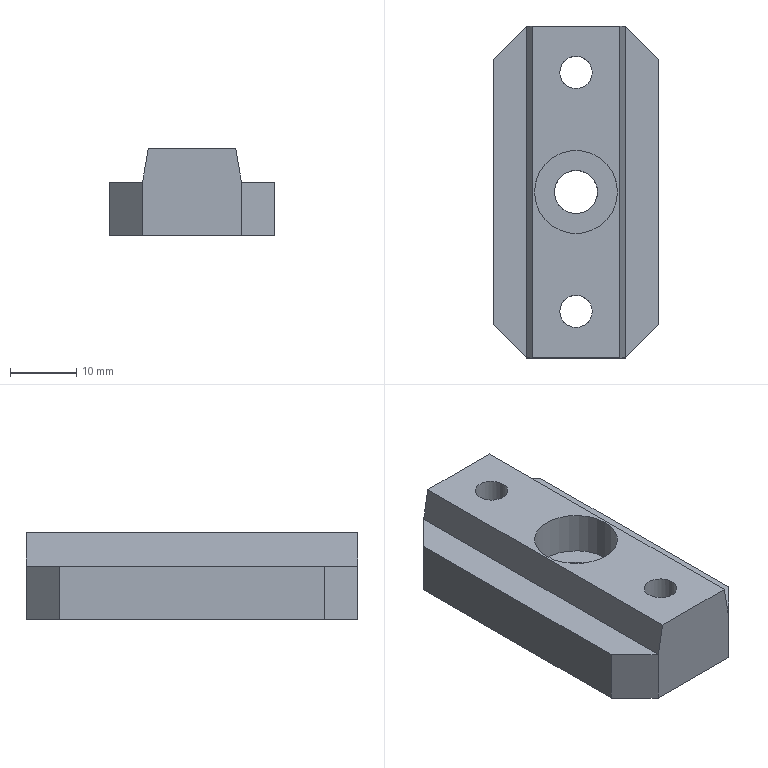Part | STEP file | 车灯-后视镜_id706_x_t | 1 solid | 19 faces | box 25 x 50 x 13 mm | volume 11607 mm3 | plane 15 | cylinder 4 | commonest cylinder face diameters 4.9 x2 6.5 x1 12.5 x1
STEP:
#1=CARTESIAN_POINT('',(-173.75,150.,4.94));
#2=VERTEX_POINT('',#1);
#3=CARTESIAN_POINT('',(-180.,150.,4.94));
#4=DIRECTION('',(0.,0.,-1.));
#5=DIRECTION('',(1.,0.,0.));
#6=AXIS2_PLACEMENT_3D('',#3,#4,#5);
#7=CIRCLE('',#6,6.25);
#8=EDGE_CURVE('',#2,#2,#7,.T.);
#9=ORIENTED_EDGE('',*,*,#8,.T.);
#10=EDGE_LOOP('',(#9));
#11=FACE_BOUND('',#10,.T.);
#12=CARTESIAN_POINT('',(-182.45,132.,4.94));
#13=VERTEX_POINT('',#12);
#14=CARTESIAN_POINT('',(-180.,132.,4.94));
#15=DIRECTION('',(0.,0.,-1.));
#16=DIRECTION('',(-1.,0.,0.));
#17=AXIS2_PLACEMENT_3D('',#14,#15,#16);
#18=CIRCLE('',#17,2.45);
#19=EDGE_CURVE('',#13,#13,#18,.T.);
#20=ORIENTED_EDGE('',*,*,#19,.T.);
#21=EDGE_LOOP('',(#20));
#22=FACE_BOUND('',#21,.T.);
#23=CARTESIAN_POINT('',(-182.45,168.,4.94));
#24=VERTEX_POINT('',#23);
#25=CARTESIAN_POINT('',(-180.,168.,4.94));
#26=DIRECTION('',(0.,0.,-1.));
#27=DIRECTION('',(-1.,0.,0.));
#28=AXIS2_PLACEMENT_3D('',#25,#26,#27);
#29=CIRCLE('',#28,2.45);
#30=EDGE_CURVE('',#24,#24,#29,.T.);
#31=ORIENTED_EDGE('',*,*,#30,.T.);
#32=EDGE_LOOP('',(#31));
#33=FACE_BOUND('',#32,.T.);
#34=CARTESIAN_POINT('',(-173.42,175.,4.94));
#35=VERTEX_POINT('',#34);
#36=CARTESIAN_POINT('',(-186.58,175.,4.94));
#37=VERTEX_POINT('',#36);
#38=CARTESIAN_POINT('',(-165.,175.,4.94));
#39=DIRECTION('',(-1.,0.,0.));
#40=VECTOR('',#39,1.);
#41=LINE('',#38,#40);
#42=EDGE_CURVE('',#35,#37,#41,.T.);
#43=ORIENTED_EDGE('',*,*,#42,.T.);
#44=CARTESIAN_POINT('',(-186.58,125.,4.94));
#45=VERTEX_POINT('',#44);
#46=CARTESIAN_POINT('',(-186.58,125.,4.94));
#47=DIRECTION('',(0.,1.,0.));
#48=VECTOR('',#47,1.);
#49=LINE('',#46,#48);
#50=EDGE_CURVE('',#45,#37,#49,.T.);
#51=ORIENTED_EDGE('',*,*,#50,.F.);
#52=CARTESIAN_POINT('',(-173.42,125.,4.94));
#53=VERTEX_POINT('',#52);
#54=CARTESIAN_POINT('',(-165.,125.,4.94));
#55=DIRECTION('',(-1.,0.,0.));
#56=VECTOR('',#55,1.);
#57=LINE('',#54,#56);
#58=EDGE_CURVE('',#53,#45,#57,.T.);
#59=ORIENTED_EDGE('',*,*,#58,.F.);
#60=CARTESIAN_POINT('',(-173.42,125.,4.94));
#61=DIRECTION('',(0.,1.,0.));
#62=VECTOR('',#61,1.);
#63=LINE('',#60,#62);
#64=EDGE_CURVE('',#53,#35,#63,.T.);
#65=ORIENTED_EDGE('',*,*,#64,.T.);
#66=EDGE_LOOP('',(#43,#51,#59,#65));
#67=FACE_BOUND('',#66,.T.);
#68=CARTESIAN_POINT('',(-172.5,125.,4.94));
#69=DIRECTION('',(0.,0.,-1.));
#70=DIRECTION('',(1.,0.,0.));
#71=AXIS2_PLACEMENT_3D('',#68,#69,#70);
#72=PLANE('',#71);
#73=ADVANCED_FACE('',(#11,#22,#33,#67),#72,.F.);
#74=CARTESIAN_POINT('',(-180.,153.25,-8.06));
#75=VERTEX_POINT('',#74);
#76=CARTESIAN_POINT('',(-180.,150.,-8.06));
#77=DIRECTION('',(0.,0.,-1.));
#78=DIRECTION('',(0.,1.,0.));
#79=AXIS2_PLACEMENT_3D('',#76,#77,#78);
#80=CIRCLE('',#79,3.25);
#81=EDGE_CURVE('',#75,#75,#80,.T.);
#82=ORIENTED_EDGE('',*,*,#81,.F.);
#83=EDGE_LOOP('',(#82));
#84=FACE_BOUND('',#83,.T.);
#85=CARTESIAN_POINT('',(-172.5,125.,-8.06));
#86=VERTEX_POINT('',#85);
#87=CARTESIAN_POINT('',(-187.5,125.,-8.06));
#88=VERTEX_POINT('',#87);
#89=CARTESIAN_POINT('',(-195.,125.,-8.06));
#90=DIRECTION('',(-1.,0.,0.));
#91=VECTOR('',#90,1.);
#92=LINE('',#89,#91);
#93=EDGE_CURVE('',#86,#88,#92,.T.);
#94=ORIENTED_EDGE('',*,*,#93,.T.);
#95=CARTESIAN_POINT('',(-192.5,130.,-8.06));
#96=VERTEX_POINT('',#95);
#97=CARTESIAN_POINT('',(-187.5,125.,-8.06));
#98=DIRECTION('',(-0.7071,0.7071,0.));
#99=VECTOR('',#98,1.);
#100=LINE('',#97,#99);
#101=EDGE_CURVE('',#88,#96,#100,.T.);
#102=ORIENTED_EDGE('',*,*,#101,.T.);
#103=CARTESIAN_POINT('',(-192.5,170.,-8.06));
#104=VERTEX_POINT('',#103);
#105=CARTESIAN_POINT('',(-192.5,100.,-8.06));
#106=DIRECTION('',(0.,-1.,0.));
#107=VECTOR('',#106,1.);
#108=LINE('',#105,#107);
#109=EDGE_CURVE('',#104,#96,#108,.T.);
#110=ORIENTED_EDGE('',*,*,#109,.F.);
#111=CARTESIAN_POINT('',(-187.5,175.,-8.06));
#112=VERTEX_POINT('',#111);
#113=CARTESIAN_POINT('',(-192.5,170.,-8.06));
#114=DIRECTION('',(0.7071,0.7071,0.));
#115=VECTOR('',#114,1.);
#116=LINE('',#113,#115);
#117=EDGE_CURVE('',#104,#112,#116,.T.);
#118=ORIENTED_EDGE('',*,*,#117,.T.);
#119=CARTESIAN_POINT('',(-172.5,175.,-8.06));
#120=VERTEX_POINT('',#119);
#121=CARTESIAN_POINT('',(-195.,175.,-8.06));
#122=DIRECTION('',(-1.,0.,0.));
#123=VECTOR('',#122,1.);
#124=LINE('',#121,#123);
#125=EDGE_CURVE('',#120,#112,#124,.T.);
#126=ORIENTED_EDGE('',*,*,#125,.F.);
#127=CARTESIAN_POINT('',(-167.5,170.,-8.06));
#128=VERTEX_POINT('',#127);
#129=CARTESIAN_POINT('',(-172.5,175.,-8.06));
#130=DIRECTION('',(0.7071,-0.7071,0.));
#131=VECTOR('',#130,1.);
#132=LINE('',#129,#131);
#133=EDGE_CURVE('',#120,#128,#132,.T.);
#134=ORIENTED_EDGE('',*,*,#133,.T.);
#135=CARTESIAN_POINT('',(-167.5,130.,-8.06));
#136=VERTEX_POINT('',#135);
#137=CARTESIAN_POINT('',(-167.5,100.,-8.06));
#138=DIRECTION('',(0.,-1.,0.));
#139=VECTOR('',#138,1.);
#140=LINE('',#137,#139);
#141=EDGE_CURVE('',#128,#136,#140,.T.);
#142=ORIENTED_EDGE('',*,*,#141,.T.);
#143=CARTESIAN_POINT('',(-167.5,130.,-8.06));
#144=DIRECTION('',(-0.7071,-0.7071,0.));
#145=VECTOR('',#144,1.);
#146=LINE('',#143,#145);
#147=EDGE_CURVE('',#136,#86,#146,.T.);
#148=ORIENTED_EDGE('',*,*,#147,.T.);
#149=EDGE_LOOP('',(#94,#102,#110,#118,#126,#134,#142,#148));
#150=FACE_BOUND('',#149,.T.);
#151=CARTESIAN_POINT('',(-180.,170.45,-8.06));
#152=VERTEX_POINT('',#151);
#153=CARTESIAN_POINT('',(-180.,168.,-8.06));
#154=DIRECTION('',(0.,0.,-1.));
#155=DIRECTION('',(0.,1.,0.));
#156=AXIS2_PLACEMENT_3D('',#153,#154,#155);
#157=CIRCLE('',#156,2.45);
#158=EDGE_CURVE('',#152,#152,#157,.T.);
#159=ORIENTED_EDGE('',*,*,#158,.F.);
#160=EDGE_LOOP('',(#159));
#161=FACE_BOUND('',#160,.T.);
#162=CARTESIAN_POINT('',(-180.,134.45,-8.06));
#163=VERTEX_POINT('',#162);
#164=CARTESIAN_POINT('',(-180.,132.,-8.06));
#165=DIRECTION('',(0.,0.,-1.));
#166=DIRECTION('',(0.,1.,0.));
#167=AXIS2_PLACEMENT_3D('',#164,#165,#166);
#168=CIRCLE('',#167,2.45);
#169=EDGE_CURVE('',#163,#163,#168,.T.);
#170=ORIENTED_EDGE('',*,*,#169,.F.);
#171=EDGE_LOOP('',(#170));
#172=FACE_BOUND('',#171,.T.);
#173=CARTESIAN_POINT('',(-195.,100.,-8.06));
#174=DIRECTION('',(0.,0.,1.));
#175=DIRECTION('',(0.,-1.,0.));
#176=AXIS2_PLACEMENT_3D('',#173,#174,#175);
#177=PLANE('',#176);
#178=ADVANCED_FACE('',(#84,#150,#161,#172),#177,.F.);
#179=CARTESIAN_POINT('',(-192.5,170.,-0.05985));
#180=VERTEX_POINT('',#179);
#181=CARTESIAN_POINT('',(-192.5,130.,-0.05985));
#182=VERTEX_POINT('',#181);
#183=CARTESIAN_POINT('',(-192.5,100.,-0.05985));
#184=DIRECTION('',(0.,-1.,0.));
#185=VECTOR('',#184,1.);
#186=LINE('',#183,#185);
#187=EDGE_CURVE('',#180,#182,#186,.T.);
#188=ORIENTED_EDGE('',*,*,#187,.T.);
#189=CARTESIAN_POINT('',(-187.5,125.,-0.05985));
#190=VERTEX_POINT('',#189);
#191=CARTESIAN_POINT('',(-178.75,116.25,-0.05985));
#192=DIRECTION('',(0.7071,-0.7071,0.));
#193=VECTOR('',#192,1.);
#194=LINE('',#191,#193);
#195=EDGE_CURVE('',#182,#190,#194,.T.);
#196=ORIENTED_EDGE('',*,*,#195,.T.);
#197=CARTESIAN_POINT('',(-187.461,125.,-0.05985));
#198=VERTEX_POINT('',#197);
#199=CARTESIAN_POINT('',(-195.,125.,-0.05985));
#200=DIRECTION('',(-1.,0.,0.));
#201=VECTOR('',#200,1.);
#202=LINE('',#199,#201);
#203=EDGE_CURVE('',#198,#190,#202,.T.);
#204=ORIENTED_EDGE('',*,*,#203,.F.);
#205=CARTESIAN_POINT('',(-187.461,175.,-0.05985));
#206=VERTEX_POINT('',#205);
#207=CARTESIAN_POINT('',(-187.461,200.,-0.05985));
#208=DIRECTION('',(0.,1.,0.));
#209=VECTOR('',#208,1.);
#210=LINE('',#207,#209);
#211=EDGE_CURVE('',#198,#206,#210,.T.);
#212=ORIENTED_EDGE('',*,*,#211,.T.);
#213=CARTESIAN_POINT('',(-187.5,175.,-0.05985));
#214=VERTEX_POINT('',#213);
#215=CARTESIAN_POINT('',(-195.,175.,-0.05985));
#216=DIRECTION('',(-1.,0.,0.));
#217=VECTOR('',#216,1.);
#218=LINE('',#215,#217);
#219=EDGE_CURVE('',#206,#214,#218,.T.);
#220=ORIENTED_EDGE('',*,*,#219,.T.);
#221=CARTESIAN_POINT('',(-228.75,133.75,-0.05985));
#222=DIRECTION('',(-0.7071,-0.7071,0.));
#223=VECTOR('',#222,1.);
#224=LINE('',#221,#223);
#225=EDGE_CURVE('',#214,#180,#224,.T.);
#226=ORIENTED_EDGE('',*,*,#225,.T.);
#227=EDGE_LOOP('',(#188,#196,#204,#212,#220,#226));
#228=FACE_OUTER_BOUND('',#227,.T.);
#229=CARTESIAN_POINT('',(-195.,100.,-0.05985));
#230=DIRECTION('',(0.,0.,1.));
#231=DIRECTION('',(0.,-1.,0.));
#232=AXIS2_PLACEMENT_3D('',#229,#230,#231);
#233=PLANE('',#232);
#234=ADVANCED_FACE('',(#228),#233,.T.);
#235=ORIENTED_EDGE('',*,*,#203,.T.);
#236=CARTESIAN_POINT('',(-187.5,125.,-8.06));
#237=DIRECTION('',(0.,0.,-1.));
#238=VECTOR('',#237,1.);
#239=LINE('',#236,#238);
#240=EDGE_CURVE('',#190,#88,#239,.T.);
#241=ORIENTED_EDGE('',*,*,#240,.T.);
#242=ORIENTED_EDGE('',*,*,#93,.F.);
#243=CARTESIAN_POINT('',(-172.5,125.,-0.05985));
#244=VERTEX_POINT('',#243);
#245=CARTESIAN_POINT('',(-172.5,125.,-10.06));
#246=DIRECTION('',(0.,0.,1.));
#247=VECTOR('',#246,1.);
#248=LINE('',#245,#247);
#249=EDGE_CURVE('',#86,#244,#248,.T.);
#250=ORIENTED_EDGE('',*,*,#249,.T.);
#251=CARTESIAN_POINT('',(-172.539,125.,-0.05985));
#252=VERTEX_POINT('',#251);
#253=CARTESIAN_POINT('',(-195.,125.,-0.05985));
#254=DIRECTION('',(-1.,0.,0.));
#255=VECTOR('',#254,1.);
#256=LINE('',#253,#255);
#257=EDGE_CURVE('',#244,#252,#256,.T.);
#258=ORIENTED_EDGE('',*,*,#257,.T.);
#259=CARTESIAN_POINT('',(-172.462,125.,-0.494));
#260=DIRECTION('',(0.1736,0.,-0.9848));
#261=VECTOR('',#260,1.);
#262=LINE('',#259,#261);
#263=EDGE_CURVE('',#53,#252,#262,.T.);
#264=ORIENTED_EDGE('',*,*,#263,.F.);
#265=ORIENTED_EDGE('',*,*,#58,.T.);
#266=CARTESIAN_POINT('',(-187.538,125.,-0.494));
#267=DIRECTION('',(-0.1736,0.,-0.9848));
#268=VECTOR('',#267,1.);
#269=LINE('',#266,#268);
#270=EDGE_CURVE('',#45,#198,#269,.T.);
#271=ORIENTED_EDGE('',*,*,#270,.T.);
#272=EDGE_LOOP('',(#235,#241,#242,#250,#258,#264,#265,#271));
#273=FACE_OUTER_BOUND('',#272,.T.);
#274=CARTESIAN_POINT('',(-165.,125.,-10.06));
#275=DIRECTION('',(0.,1.,0.));
#276=DIRECTION('',(1.,0.,0.));
#277=AXIS2_PLACEMENT_3D('',#274,#275,#276);
#278=PLANE('',#277);
#279=ADVANCED_FACE('',(#273),#278,.F.);
#280=ORIENTED_EDGE('',*,*,#109,.T.);
#281=CARTESIAN_POINT('',(-192.5,130.,-0.05985));
#282=DIRECTION('',(0.,0.,1.));
#283=VECTOR('',#282,1.);
#284=LINE('',#281,#283);
#285=EDGE_CURVE('',#96,#182,#284,.T.);
#286=ORIENTED_EDGE('',*,*,#285,.T.);
#287=ORIENTED_EDGE('',*,*,#187,.F.);
#288=CARTESIAN_POINT('',(-192.5,170.,-10.06));
#289=DIRECTION('',(0.,0.,-1.));
#290=VECTOR('',#289,1.);
#291=LINE('',#288,#290);
#292=EDGE_CURVE('',#180,#104,#291,.T.);
#293=ORIENTED_EDGE('',*,*,#292,.T.);
#294=EDGE_LOOP('',(#280,#286,#287,#293));
#295=FACE_OUTER_BOUND('',#294,.T.);
#296=CARTESIAN_POINT('',(-192.5,200.,-10.06));
#297=DIRECTION('',(-1.,0.,0.));
#298=DIRECTION('',(0.,1.,0.));
#299=AXIS2_PLACEMENT_3D('',#296,#297,#298);
#300=PLANE('',#299);
#301=ADVANCED_FACE('',(#295),#300,.T.);
#302=CARTESIAN_POINT('',(-172.5,175.,-0.05985));
#303=VERTEX_POINT('',#302);
#304=CARTESIAN_POINT('',(-172.539,175.,-0.05985));
#305=VERTEX_POINT('',#304);
#306=CARTESIAN_POINT('',(-195.,175.,-0.05985));
#307=DIRECTION('',(-1.,0.,0.));
#308=VECTOR('',#307,1.);
#309=LINE('',#306,#308);
#310=EDGE_CURVE('',#303,#305,#309,.T.);
#311=ORIENTED_EDGE('',*,*,#310,.F.);
#312=CARTESIAN_POINT('',(-172.5,175.,-8.06));
#313=DIRECTION('',(0.,0.,-1.));
#314=VECTOR('',#313,1.);
#315=LINE('',#312,#314);
#316=EDGE_CURVE('',#303,#120,#315,.T.);
#317=ORIENTED_EDGE('',*,*,#316,.T.);
#318=ORIENTED_EDGE('',*,*,#125,.T.);
#319=CARTESIAN_POINT('',(-187.5,175.,-10.06));
#320=DIRECTION('',(0.,0.,1.));
#321=VECTOR('',#320,1.);
#322=LINE('',#319,#321);
#323=EDGE_CURVE('',#112,#214,#322,.T.);
#324=ORIENTED_EDGE('',*,*,#323,.T.);
#325=ORIENTED_EDGE('',*,*,#219,.F.);
#326=CARTESIAN_POINT('',(-187.538,175.,-0.494));
#327=DIRECTION('',(-0.1736,0.,-0.9848));
#328=VECTOR('',#327,1.);
#329=LINE('',#326,#328);
#330=EDGE_CURVE('',#37,#206,#329,.T.);
#331=ORIENTED_EDGE('',*,*,#330,.F.);
#332=ORIENTED_EDGE('',*,*,#42,.F.);
#333=CARTESIAN_POINT('',(-172.462,175.,-0.494));
#334=DIRECTION('',(0.1736,0.,-0.9848));
#335=VECTOR('',#334,1.);
#336=LINE('',#333,#335);
#337=EDGE_CURVE('',#35,#305,#336,.T.);
#338=ORIENTED_EDGE('',*,*,#337,.T.);
#339=EDGE_LOOP('',(#311,#317,#318,#324,#325,#331,#332,#338));
#340=FACE_OUTER_BOUND('',#339,.T.);
#341=CARTESIAN_POINT('',(-165.,175.,-10.06));
#342=DIRECTION('',(0.,1.,0.));
#343=DIRECTION('',(1.,0.,0.));
#344=AXIS2_PLACEMENT_3D('',#341,#342,#343);
#345=PLANE('',#344);
#346=ADVANCED_FACE('',(#340),#345,.T.);
#347=CARTESIAN_POINT('',(-167.5,170.,-0.05985));
#348=VERTEX_POINT('',#347);
#349=CARTESIAN_POINT('',(-167.5,130.,-0.05985));
#350=VERTEX_POINT('',#349);
#351=CARTESIAN_POINT('',(-167.5,100.,-0.05985));
#352=DIRECTION('',(0.,-1.,0.));
#353=VECTOR('',#352,1.);
#354=LINE('',#351,#353);
#355=EDGE_CURVE('',#348,#350,#354,.T.);
#356=ORIENTED_EDGE('',*,*,#355,.T.);
#357=CARTESIAN_POINT('',(-167.5,130.,-10.06));
#358=DIRECTION('',(0.,0.,-1.));
#359=VECTOR('',#358,1.);
#360=LINE('',#357,#359);
#361=EDGE_CURVE('',#350,#136,#360,.T.);
#362=ORIENTED_EDGE('',*,*,#361,.T.);
#363=ORIENTED_EDGE('',*,*,#141,.F.);
#364=CARTESIAN_POINT('',(-167.5,170.,-0.05985));
#365=DIRECTION('',(0.,0.,1.));
#366=VECTOR('',#365,1.);
#367=LINE('',#364,#366);
#368=EDGE_CURVE('',#128,#348,#367,.T.);
#369=ORIENTED_EDGE('',*,*,#368,.T.);
#370=EDGE_LOOP('',(#356,#362,#363,#369));
#371=FACE_OUTER_BOUND('',#370,.T.);
#372=CARTESIAN_POINT('',(-167.5,200.,-10.06));
#373=DIRECTION('',(-1.,0.,0.));
#374=DIRECTION('',(0.,1.,0.));
#375=AXIS2_PLACEMENT_3D('',#372,#373,#374);
#376=PLANE('',#375);
#377=ADVANCED_FACE('',(#371),#376,.F.);
#378=ORIENTED_EDGE('',*,*,#257,.F.);
#379=CARTESIAN_POINT('',(-196.25,101.25,-0.05985));
#380=DIRECTION('',(0.7071,0.7071,0.));
#381=VECTOR('',#380,1.);
#382=LINE('',#379,#381);
#383=EDGE_CURVE('',#244,#350,#382,.T.);
#384=ORIENTED_EDGE('',*,*,#383,.T.);
#385=ORIENTED_EDGE('',*,*,#355,.F.);
#386=CARTESIAN_POINT('',(-146.25,148.75,-0.05985));
#387=DIRECTION('',(-0.7071,0.7071,0.));
#388=VECTOR('',#387,1.);
#389=LINE('',#386,#388);
#390=EDGE_CURVE('',#348,#303,#389,.T.);
#391=ORIENTED_EDGE('',*,*,#390,.T.);
#392=ORIENTED_EDGE('',*,*,#310,.T.);
#393=CARTESIAN_POINT('',(-172.539,200.,-0.05985));
#394=DIRECTION('',(0.,1.,0.));
#395=VECTOR('',#394,1.);
#396=LINE('',#393,#395);
#397=EDGE_CURVE('',#252,#305,#396,.T.);
#398=ORIENTED_EDGE('',*,*,#397,.F.);
#399=EDGE_LOOP('',(#378,#384,#385,#391,#392,#398));
#400=FACE_OUTER_BOUND('',#399,.T.);
#401=CARTESIAN_POINT('',(-195.,100.,-0.05985));
#402=DIRECTION('',(0.,0.,1.));
#403=DIRECTION('',(0.,-1.,0.));
#404=AXIS2_PLACEMENT_3D('',#401,#402,#403);
#405=PLANE('',#404);
#406=ADVANCED_FACE('',(#400),#405,.T.);
#407=ORIENTED_EDGE('',*,*,#397,.T.);
#408=ORIENTED_EDGE('',*,*,#337,.F.);
#409=ORIENTED_EDGE('',*,*,#64,.F.);
#410=ORIENTED_EDGE('',*,*,#263,.T.);
#411=EDGE_LOOP('',(#407,#408,#409,#410));
#412=FACE_OUTER_BOUND('',#411,.T.);
#413=CARTESIAN_POINT('',(-172.462,200.,-0.494));
#414=DIRECTION('',(0.9848,0.,0.1736));
#415=DIRECTION('',(-0.1736,0.,0.9848));
#416=AXIS2_PLACEMENT_3D('',#413,#414,#415);
#417=PLANE('',#416);
#418=ADVANCED_FACE('',(#412),#417,.T.);
#419=ORIENTED_EDGE('',*,*,#211,.F.);
#420=ORIENTED_EDGE('',*,*,#270,.F.);
#421=ORIENTED_EDGE('',*,*,#50,.T.);
#422=ORIENTED_EDGE('',*,*,#330,.T.);
#423=EDGE_LOOP('',(#419,#420,#421,#422));
#424=FACE_OUTER_BOUND('',#423,.T.);
#425=CARTESIAN_POINT('',(-187.538,200.,-0.494));
#426=DIRECTION('',(-0.9848,0.,0.1736));
#427=DIRECTION('',(-0.1736,0.,-0.9848));
#428=AXIS2_PLACEMENT_3D('',#425,#426,#427);
#429=PLANE('',#428);
#430=ADVANCED_FACE('',(#424),#429,.T.);
#431=ORIENTED_EDGE('',*,*,#158,.T.);
#432=EDGE_LOOP('',(#431));
#433=FACE_BOUND('',#432,.T.);
#434=ORIENTED_EDGE('',*,*,#30,.F.);
#435=EDGE_LOOP('',(#434));
#436=FACE_BOUND('',#435,.T.);
#437=CARTESIAN_POINT('',(-180.,168.,-10.06));
#438=DIRECTION('',(0.,0.,1.));
#439=DIRECTION('',(-1.,0.,0.));
#440=AXIS2_PLACEMENT_3D('',#437,#438,#439);
#441=CYLINDRICAL_SURFACE('',#440,2.45);
#442=ADVANCED_FACE('',(#433,#436),#441,.F.);
#443=CARTESIAN_POINT('',(-176.75,150.,-1.56));
#444=VERTEX_POINT('',#443);
#445=CARTESIAN_POINT('',(-180.,150.,-1.56));
#446=DIRECTION('',(0.,0.,-1.));
#447=DIRECTION('',(1.,0.,0.));
#448=AXIS2_PLACEMENT_3D('',#445,#446,#447);
#449=CIRCLE('',#448,3.25);
#450=EDGE_CURVE('',#444,#444,#449,.T.);
#451=ORIENTED_EDGE('',*,*,#450,.F.);
#452=EDGE_LOOP('',(#451));
#453=FACE_BOUND('',#452,.T.);
#454=ORIENTED_EDGE('',*,*,#81,.T.);
#455=EDGE_LOOP('',(#454));
#456=FACE_BOUND('',#455,.T.);
#457=CARTESIAN_POINT('',(-180.,150.,-10.06));
#458=DIRECTION('',(0.,0.,1.));
#459=DIRECTION('',(-1.,0.,0.));
#460=AXIS2_PLACEMENT_3D('',#457,#458,#459);
#461=CYLINDRICAL_SURFACE('',#460,3.25);
#462=ADVANCED_FACE('',(#453,#456),#461,.F.);
#463=ORIENTED_EDGE('',*,*,#169,.T.);
#464=EDGE_LOOP('',(#463));
#465=FACE_BOUND('',#464,.T.);
#466=ORIENTED_EDGE('',*,*,#19,.F.);
#467=EDGE_LOOP('',(#466));
#468=FACE_BOUND('',#467,.T.);
#469=CARTESIAN_POINT('',(-180.,132.,-10.06));
#470=DIRECTION('',(0.,0.,1.));
#471=DIRECTION('',(-1.,0.,0.));
#472=AXIS2_PLACEMENT_3D('',#469,#470,#471);
#473=CYLINDRICAL_SURFACE('',#472,2.45);
#474=ADVANCED_FACE('',(#465,#468),#473,.F.);
#475=CARTESIAN_POINT('',(-173.75,150.,-1.56));
#476=VERTEX_POINT('',#475);
#477=CARTESIAN_POINT('',(-180.,150.,-1.56));
#478=DIRECTION('',(0.,0.,-1.));
#479=DIRECTION('',(1.,0.,0.));
#480=AXIS2_PLACEMENT_3D('',#477,#478,#479);
#481=CIRCLE('',#480,6.25);
#482=EDGE_CURVE('',#476,#476,#481,.T.);
#483=ORIENTED_EDGE('',*,*,#482,.T.);
#484=EDGE_LOOP('',(#483));
#485=FACE_BOUND('',#484,.T.);
#486=ORIENTED_EDGE('',*,*,#8,.F.);
#487=EDGE_LOOP('',(#486));
#488=FACE_BOUND('',#487,.T.);
#489=CARTESIAN_POINT('',(-180.,150.,-1.56));
#490=DIRECTION('',(0.,0.,1.));
#491=DIRECTION('',(-1.,0.,0.));
#492=AXIS2_PLACEMENT_3D('',#489,#490,#491);
#493=CYLINDRICAL_SURFACE('',#492,6.25);
#494=ADVANCED_FACE('',(#485,#488),#493,.F.);
#495=ORIENTED_EDGE('',*,*,#450,.T.);
#496=EDGE_LOOP('',(#495));
#497=FACE_BOUND('',#496,.T.);
#498=ORIENTED_EDGE('',*,*,#482,.F.);
#499=EDGE_LOOP('',(#498));
#500=FACE_BOUND('',#499,.T.);
#501=CARTESIAN_POINT('',(-180.,150.,-1.56));
#502=DIRECTION('',(0.,0.,-1.));
#503=DIRECTION('',(1.,0.,0.));
#504=AXIS2_PLACEMENT_3D('',#501,#502,#503);
#505=PLANE('',#504);
#506=ADVANCED_FACE('',(#497,#500),#505,.F.);
#507=ORIENTED_EDGE('',*,*,#195,.F.);
#508=ORIENTED_EDGE('',*,*,#285,.F.);
#509=ORIENTED_EDGE('',*,*,#101,.F.);
#510=ORIENTED_EDGE('',*,*,#240,.F.);
#511=EDGE_LOOP('',(#507,#508,#509,#510));
#512=FACE_OUTER_BOUND('',#511,.T.);
#513=CARTESIAN_POINT('',(-187.5,125.,-10.06));
#514=DIRECTION('',(-0.7071,-0.7071,0.));
#515=DIRECTION('',(-0.7071,0.7071,0.));
#516=AXIS2_PLACEMENT_3D('',#513,#514,#515);
#517=PLANE('',#516);
#518=ADVANCED_FACE('',(#512),#517,.T.);
#519=ORIENTED_EDGE('',*,*,#383,.F.);
#520=ORIENTED_EDGE('',*,*,#249,.F.);
#521=ORIENTED_EDGE('',*,*,#147,.F.);
#522=ORIENTED_EDGE('',*,*,#361,.F.);
#523=EDGE_LOOP('',(#519,#520,#521,#522));
#524=FACE_OUTER_BOUND('',#523,.T.);
#525=CARTESIAN_POINT('',(-167.5,130.,-10.06));
#526=DIRECTION('',(-0.7071,0.7071,0.));
#527=DIRECTION('',(0.7071,0.7071,0.));
#528=AXIS2_PLACEMENT_3D('',#525,#526,#527);
#529=PLANE('',#528);
#530=ADVANCED_FACE('',(#524),#529,.F.);
#531=ORIENTED_EDGE('',*,*,#390,.F.);
#532=ORIENTED_EDGE('',*,*,#368,.F.);
#533=ORIENTED_EDGE('',*,*,#133,.F.);
#534=ORIENTED_EDGE('',*,*,#316,.F.);
#535=EDGE_LOOP('',(#531,#532,#533,#534));
#536=FACE_OUTER_BOUND('',#535,.T.);
#537=CARTESIAN_POINT('',(-172.5,175.,-10.06));
#538=DIRECTION('',(0.7071,0.7071,0.));
#539=DIRECTION('',(0.7071,-0.7071,0.));
#540=AXIS2_PLACEMENT_3D('',#537,#538,#539);
#541=PLANE('',#540);
#542=ADVANCED_FACE('',(#536),#541,.T.);
#543=ORIENTED_EDGE('',*,*,#225,.F.);
#544=ORIENTED_EDGE('',*,*,#323,.F.);
#545=ORIENTED_EDGE('',*,*,#117,.F.);
#546=ORIENTED_EDGE('',*,*,#292,.F.);
#547=EDGE_LOOP('',(#543,#544,#545,#546));
#548=FACE_OUTER_BOUND('',#547,.T.);
#549=CARTESIAN_POINT('',(-192.5,170.,-10.06));
#550=DIRECTION('',(0.7071,-0.7071,0.));
#551=DIRECTION('',(-0.7071,-0.7071,0.));
#552=AXIS2_PLACEMENT_3D('',#549,#550,#551);
#553=PLANE('',#552);
#554=ADVANCED_FACE('',(#548),#553,.F.);
#555=CLOSED_SHELL('',(#73,#178,#234,#279,#301,#346,#377,#406,#418,#430,#442,#462,#474,#494,#506,#518,#530,#542,#554));
#556=MANIFOLD_SOLID_BREP('',#555);
#557=(LENGTH_UNIT()NAMED_UNIT(*)SI_UNIT(.MILLI.,.METRE.));
#558=UNCERTAINTY_MEASURE_WITH_UNIT(LENGTH_MEASURE(0.00002),#557,'','');
#559=(NAMED_UNIT(*)PLANE_ANGLE_UNIT()SI_UNIT($,.RADIAN.));
#560=PLANE_ANGLE_MEASURE_WITH_UNIT(PLANE_ANGLE_MEASURE(0.01745),#559);
#561=DIMENSIONAL_EXPONENTS(0.,0.,0.,0.,0.,0.,0.);
#562=(CONVERSION_BASED_UNIT('DEGREE',#560)NAMED_UNIT(#561)PLANE_ANGLE_UNIT());
#563=(NAMED_UNIT(*)SI_UNIT($,.STERADIAN.)SOLID_ANGLE_UNIT());
#564=(GEOMETRIC_REPRESENTATION_CONTEXT(3)GLOBAL_UNCERTAINTY_ASSIGNED_CONTEXT((#558))GLOBAL_UNIT_ASSIGNED_CONTEXT((#557,#562,#563))REPRESENTATION_CONTEXT('',''));
#565=ADVANCED_BREP_SHAPE_REPRESENTATION('',(#556),#564);